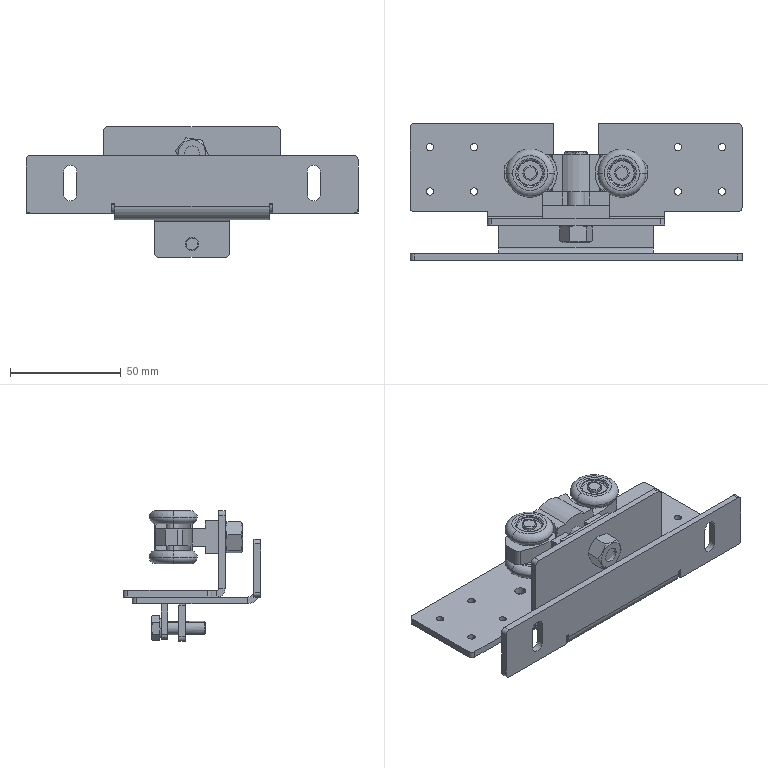Part | NX | features BREP 6 | 6 solids | 394 faces | box 150 x 62 x 59 mm | volume 71777 mm3 | plane 168 | cylinder 148 | torus 60 | cone 18 | commonest cylinder face diameters 4 x22 12 x17 1 x16 3.3 x16 6.5 x16 5 x8